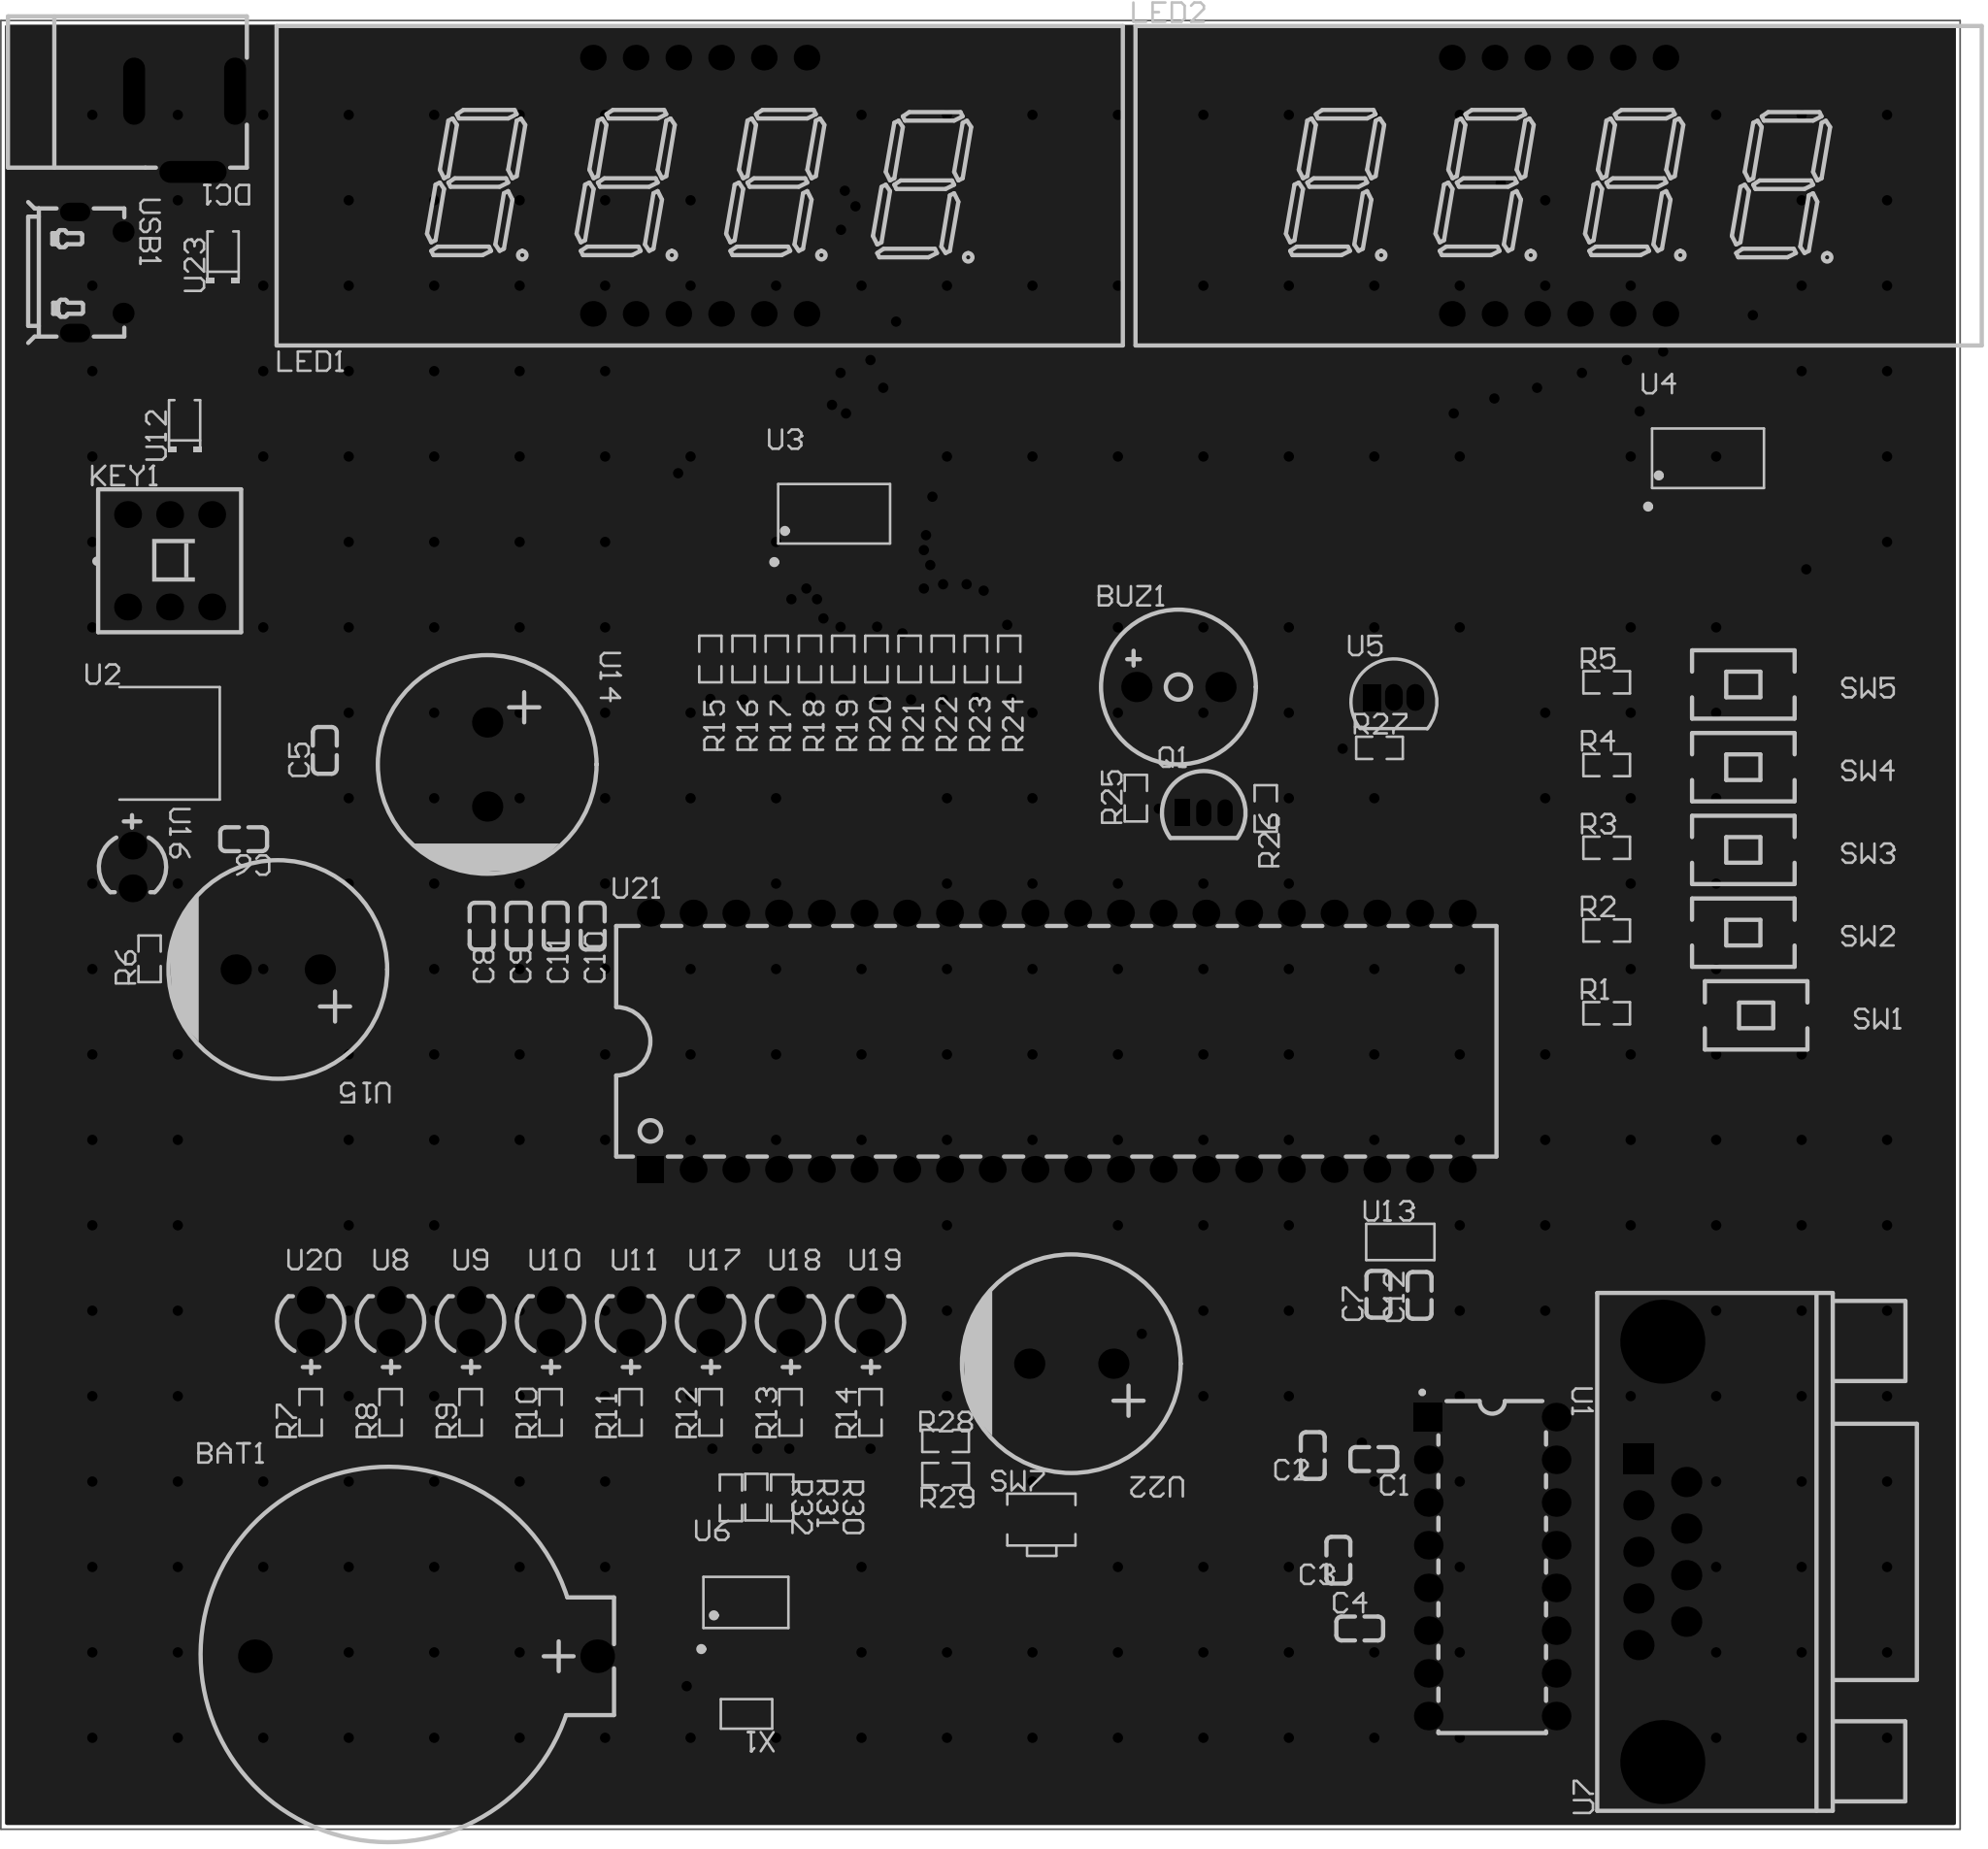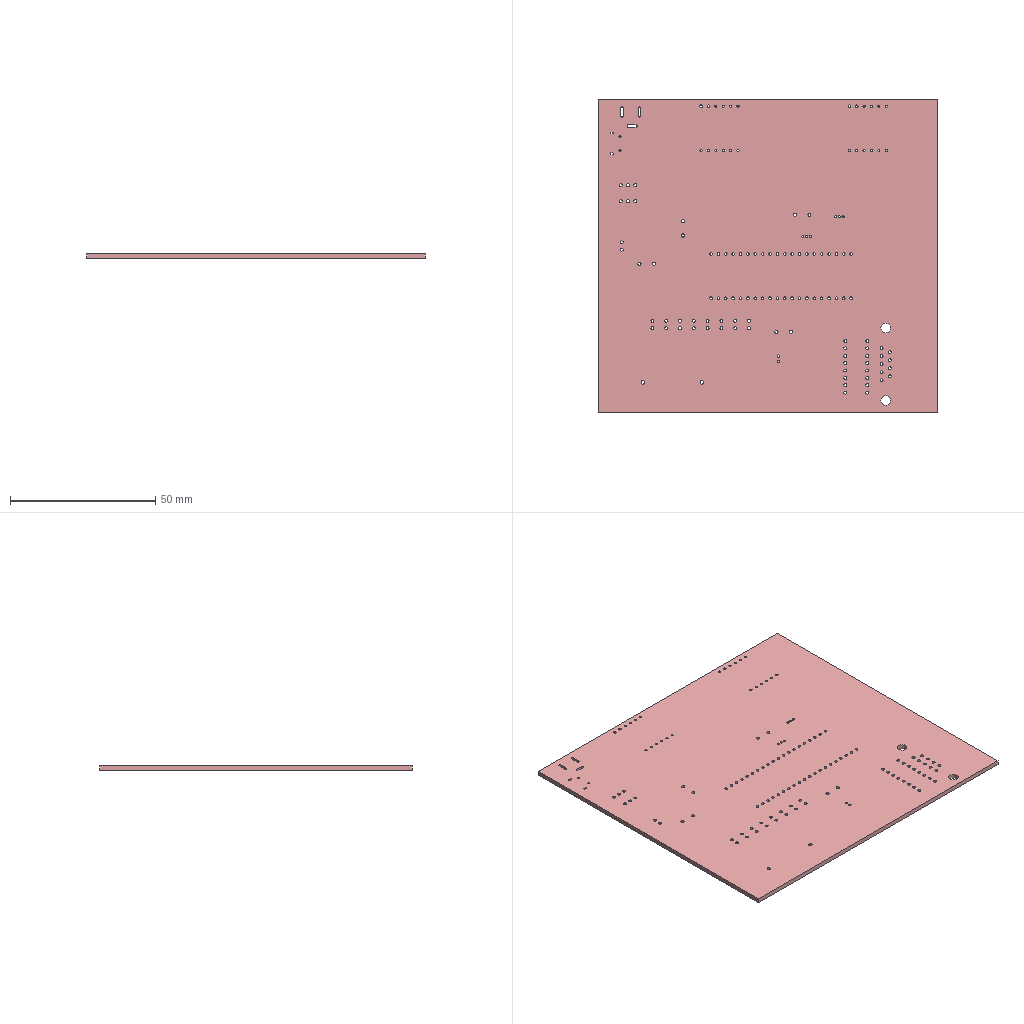Circuit board layout | Altium Designer | box 116.5 x 107.6 x 1.6 mm
Layer stack:
# Altium Designer layer stack of  (unit mm; dielectric type: 0 none, 1 core, 2 prepreg, 3 surface material)
index,name,kind,layer,copper_thickness_mm,dielectric_type,dielectric_thickness_mm,dielectric_material,dielectric_constant
0,Top Paste Mask Layer,other,,,,,,
1,Top Silkscreen Layer,other,,,,,,
2,Top Solder Mask Layer,dielectric,,,3,0.01,,3.3
3,Top Layer,copper,Top Layer,0.035,,,,
4,Dielectric1,dielectric,,,3,1.51,FR4,4.5
5,Bottom Layer,copper,Bottom Layer,0.035,,,,
6,Bottom Solder Mask Layer,dielectric,,,3,0.01,,3.3
7,Bottom Silkscreen Layer,other,,,,,,
8,Bottom Paste Mask Layer,other,,,,,,
# drill layer pairs: low layer,high layer
drill_pair,Top Layer,Bottom Layer
Part placement:
Designator,Comment,Layer,Footprint,Center-X(mm),Center-Y(mm),Rotation
BUZ1,Buzzer,TopLayer,BUZ-TH_BD9.0-P5.00-D0.6-FD,160.419,151.371,0
C1,104,TopLayer,C0603,172.032,105.452,180
C2,4.7uF,TopLayer,C0603,168.402,105.664,90
C3,4.7uF,TopLayer,C0603,169.926,99.441,90
C4,4.7uF,TopLayer,C0603,171.196,95.377,0
C5,4.7uF,TopLayer,C0603,109.68,147.6,90
C6,4.7uF,TopLayer,C0603,104.857,142.317,180
C7,100nF,TopLayer,C0603,172.308,115.254,90
C8,4.7uF,TopLayer,C0603,118.999,137.15,90
C9,4.7uF,TopLayer,C0603,121.2,137.15,90
C10,4.7uF,TopLayer,C0603,125.603,137.15,90
C11,4.7uF,TopLayer,C0603,123.402,137.15,90
C12,100nF,TopLayer,C0603,174.752,115.189,90
LED1,FJ5461AB,TopLayer,LED-SEG-TH_12P-L50.4-W19.0-P2.54-S15.24-BL,131.964,181.182,0
LED2,FJ5461AB,TopLayer,LED-SEG-TH_12P-L50.4-W19.0-P2.54-S15.24-BL,183.018,181.182,0
Q1,2SC945,TopLayer,TO-92-3_L4.9-W3.7-P1.27-L,161.925,143.891,0
R1,48.7Ω,TopLayer,R0603,185.875,131.969,0
R2,48.7Ω,TopLayer,R0603,185.875,136.888,0
R3,48.7Ω,TopLayer,R0603,185.875,141.808,0
R4,48.7Ω,TopLayer,R0603,185.875,146.728,0
R5,48.7Ω,TopLayer,R0603,185.875,151.648,0
R6,10K,TopLayer,R0603,99.266,135.205,90
R7,10K,TopLayer,R0603,108.837,108.233,90
R8,10K,TopLayer,R0603,113.591,108.233,90
R9,10K,TopLayer,R0603,118.345,108.233,90
R10,10K,TopLayer,R0603,123.099,108.233,90
R11,10K,TopLayer,R0603,127.853,108.233,90
R12,10K,TopLayer,R0603,132.607,108.233,90
R13,10K,TopLayer,R0603,137.361,108.233,90
R14,10K,TopLayer,R0603,142.115,108.233,90
R15,10K,TopLayer,R0603,132.597,153.035,90
R16,10K,TopLayer,R0603,134.57,153.035,90
R17,10K,TopLayer,R0603,136.544,153.035,90
R18,10K,TopLayer,R0603,138.518,153.035,90
R19,10K,TopLayer,R0603,140.491,153.035,90
R20,10K,TopLayer,R0603,142.465,153.035,90
R21,10K,TopLayer,R0603,144.438,153.035,90
R22,10K,TopLayer,R0603,146.412,153.035,90
R23,10K,TopLayer,R0603,148.386,153.035,90
R24,10K,TopLayer,R0603,150.359,153.035,90
R25,50,TopLayer,R0603,157.888,144.759,90
R26,1K,TopLayer,R0603,165.608,144.145,90
R27,10K,TopLayer,R0603,172.371,147.751,0
R28,10K,TopLayer,R0603,146.578,106.535,180
R29,10K,TopLayer,R0603,146.578,104.562,0
SW1,SW_PB_ESW_1,TopLayer,KEY-SMD_L6.1-W3.8-LS8.0,194.758,131.841,0
SW2,SW_PB_ESW_1,TopLayer,KEY-SMD_L6.1-W3.8-LS8.0,193.996,136.761,0
SW3,SW_PB_ESW_1,TopLayer,KEY-SMD_L6.1-W3.8-LS8.0,193.996,141.681,0
SW4,SW_PB_ESW_1,TopLayer,KEY-SMD_L6.1-W3.8-LS8.0,193.996,146.601,0
SW5,SW_PB_ESW_1,TopLayer,KEY-SMD_L6.1-W3.8-LS8.0,193.996,151.521,0
SW7,YD-3410,TopLayer,SW-SMD_L3.9-W2.9-LS4.8-EH-A,152.273,101.854,0
U1,MAX232AEJE,TopLayer,PDIP-16_L19.3-W6.5-P2.54-LS7.6-BL,179.07,99.06,270
U2,LM1117IDT-5.0,TopLayer,TO-252-2_L6.6-W6.1-P4.57-LS9.7-BR-CW,102.055,148.018,0
U3,74HC573PW/AU118,TopLayer,TSSOP-20_L6.5-W4.4-P0.65-LS6.4-BL,139.954,161.671,0
U4,74HC573PW/AU118,TopLayer,TSSOP-20_L6.5-W4.4-P0.65-LS6.4-BL,191.897,164.973,0
U5,DS18B20+T&R-HX,TopLayer,TO-92-3_L5.1-W4.1-P1.27-L-1,173.228,150.749,0
U6,DS1302Z+T&R-TUDI,TopLayer,SOIC-8_L4.9-W3.9-P1.27-LS6.0-BL,134.71,96.927,0
U7,DB9F,TopLayer,DB9-TH_DB9F_C9900018961,189.182,99.934,90
U8,LED,TopLayer,LED-TH_BD4.0-P2.54-FD_RED,113.591,113.637,90
U9,LED,TopLayer,LED-TH_BD4.0-P2.54-FD_RED,118.345,113.637,90
U10,LED,TopLayer,LED-TH_BD4.0-P2.54-FD_RED,123.099,113.637,90
U11,LED,TopLayer,LED-TH_BD4.0-P2.54-FD_RED,127.853,113.637,90
U12,IN5819,TopLayer,SOD-123_L2.7-W1.7-LS3.8-RD,101.346,167.005,90
U13,2.768KHz,TopLayer,CRYSTAL-SMD_L3.2-W1.5-1,173.609,118.364,0
U14,CE63V1000uF13*25,TopLayer,CAP-TH_BD13.0-P5.00-D0.6-FD,119.332,146.762,270
U15,10uF,TopLayer,CAP-TH_BD13.0-P5.00-D0.6-FD,106.886,134.57,180
U16,LED,TopLayer,LED-TH_BD4.0-P2.54-FD_RED,98.25,140.666,270
U17,LED,TopLayer,LED-TH_BD4.0-P2.54-FD_RED,132.607,113.637,90
U18,LED,TopLayer,LED-TH_BD4.0-P2.54-FD_RED,137.361,113.637,90
U19,LED,TopLayer,LED-TH_BD4.0-P2.54-FD_RED,142.115,113.637,90
U20,LED,TopLayer,LED-TH_BD4.0-P2.54-FD_RED,108.837,113.637,90
U21,STC89C53RC-40I-PDIP40,TopLayer,DIP-40_L52.0-W13.7-P2.54-LS15.2-BL,153.162,130.302,0
U22,CE63V1000uF13*25,TopLayer,CAP-TH_BD13.0-P5.00-D0.6-FD,154.051,111.125,180
USB1,MICRO-USB-1,TopLayer,MICRO-USB-SMD_C9900008946,96.266,176.022,270
BAT1,CR2032-2-1,TopLayer,BAT-TH_CR2032-2-1,115.697,93.726,0
DC1,,TopLayer,DC-2.0,101.346,184.404,180
KEY1,Non-latching switch 8.5×8.5 silent,TopLayer,SW-TH_6P-L8.5-W8.5-P2.54,100.457,158.877,0
R30,4.7K,TopLayer,R0603,136.869,103.15,270
R31,4.7K,TopLayer,R0603,135.325,103.191,270
R32,4.7K,TopLayer,R0603,133.821,103.15,270
U23,IN5819,TopLayer,SOD-123_L2.7-W1.7-LS3.8-RD,103.632,177.038,90
X1,32.768K,TopLayer,OSC-SMD_L2.0-W1.2,134.747,90.297,180
Pad and via stacks:
# Altium Designer via and pad stacks of  (unit mm). Each distinct definition once, with the count of objects using it.
# via: kind,start_layer,end_layer,hole_mm,diameter_mm,mode(0 simple;1 top-mid-bottom;2 full stack),diameter_per_layer,count,example_net
# pad: kind,layer,hole_mm,hole_type(0 round;1 square;2 slot),plating,top_size,top_shape(1 round;2 rect;3 octagon;9 rounded rect),mid_size,bottom_size,mode,footprint,size_per_layer,count,example
pad,Multi-Layer,1,0,plated,1.8x1.8,1,1.8x1.8,1.8x1.8,0,BUZ-TH_BD9.0-P5.00-D0.6-FD,,2,BUZ1.1
pad,Multi-Layer,0.9144,0,plated,1.524x1.524,1,1.524x1.524,1.524x1.524,0,LED-SEG-TH_12P-L50.4-W19.0-P2.54-S15.24-BL,,4,LED1.12
pad,Multi-Layer,0.762,0,plated,1.524x1.524,1,1.524x1.524,1.524x1.524,0,LED-SEG-TH_12P-L50.4-W19.0-P2.54-S15.24-BL,,20,LED1.10
pad,Multi-Layer,0.7,0,plated,0.9x1.6,1,0.9x1.6,0.9x1.6,0,TO-92-3_L4.9-W3.7-P1.27-L,,2,Q1.3
pad,Multi-Layer,0.7,0,plated,0.9x1.6,2,0.9x1.6,0.9x1.6,0,TO-92-3_L4.9-W3.7-P1.27-L,,1,Q1.1
pad,Multi-Layer,1,0,plated,1.7x1.7,2,1.7x1.7,1.7x1.7,0,PDIP-16_L19.3-W6.5-P2.54-LS7.6-BL,,1,U1.1
pad,Multi-Layer,1,0,plated,1.7x1.7,1,1.7x1.7,1.7x1.7,0,PDIP-16_L19.3-W6.5-P2.54-LS7.6-BL,,15,U1.2
pad,Multi-Layer,0.75,0,plated,1.05x1.6,2,1.05x1.6,1.05x1.6,0,TO-92-3_L5.1-W4.1-P1.27-L-1,,1,U5.1
pad,Multi-Layer,0.75,0,plated,1.05x1.6,1,1.05x1.6,1.05x1.6,0,TO-92-3_L5.1-W4.1-P1.27-L-1,,2,U5.2
pad,Multi-Layer,3.25,0,plated,5x5,1,5x5,5x5,0,DB9-TH_DB9F_C9900018961,,2,U7.10
pad,Multi-Layer,1.05,0,plated,1.8x1.8,1,1.8x1.8,1.8x1.8,0,DB9-TH_DB9F_C9900018961,,8,U7.6
pad,Multi-Layer,1.05,0,plated,1.8x1.8,2,1.8x1.8,1.8x1.8,0,DB9-TH_DB9F_C9900018961,,1,U7.1
pad,Multi-Layer,1,0,plated,1.651x1.651,1,1.651x1.651,1.651x1.651,0,LED-TH_BD4.0-P2.54-FD_RED,,18,U8.2
pad,Multi-Layer,1.1,0,plated,1.8x1.8,1,1.8x1.8,1.8x1.8,0,CAP-TH_BD13.0-P5.00-D0.6-FD,,6,U14.1
pad,Multi-Layer,0.889,0,plated,1.6x1.6,1,1.6x1.6,1.6x1.6,0,DIP-40_L52.0-W13.7-P2.54-LS15.2-BL,,39,U21.31
pad,Multi-Layer,0.889,0,plated,1.6x1.6,2,1.6x1.6,1.6x1.6,0,DIP-40_L52.0-W13.7-P2.54-LS15.2-BL,,1,U21.1
pad,Multi-Layer,0.7,0,plated,1.25x1.25,1,1.25x1.25,1.25x1.25,0,MICRO-USB-SMD_C9900008946,,2,USB1.6
pad,Multi-Layer,0.6,2,plated,1.1x1.8,1,1.1x1.8,1.1x1.8,0,MICRO-USB-SMD_C9900008946,,2,USB1.6
pad,Multi-Layer,1.2,0,plated,2x2,1,2x2,2x2,0,BAT-TH_CR2032-2-1,,2,BAT1.2
pad,Multi-Layer,0.8001,2,plated,4x1.3,1,4x1.3,4x1.3,0,DC-2.0,,3,DC1.2
pad,Multi-Layer,1,0,plated,1.6x1.6,1,1.6x1.6,1.6x1.6,0,SW-TH_6P-L8.5-W8.5-P2.54,,6,KEY1.4
pad,Top Layer,0,0,plated,0.8x0.9,2,0.8x0.9,0.8x0.9,0,C0603,,24,C1.2
pad,Top Layer,0,0,plated,0.8065x0.864,2,0.8065x0.864,0.8065x0.864,0,R0603,,64,R1.2
pad,Top Layer,0,0,plated,2x1.2,2,2x1.2,2x1.2,0,KEY-SMD_L6.1-W3.8-LS8.0,,10,SW1.1
pad,Top Layer,0,0,plated,1.23x1.5,2,1.23x1.5,1.23x1.5,0,SW-SMD_L3.9-W2.9-LS4.8-EH-A,,2,SW7.2
pad,Top Layer,0,0,plated,6.2x5.8,2,6.2x5.8,6.2x5.8,0,TO-252-2_L6.6-W6.1-P4.57-LS9.7-BR-CW,,1,U2.2
pad,Top Layer,0,0,plated,3x1.6,2,3x1.6,3x1.6,0,TO-252-2_L6.6-W6.1-P4.57-LS9.7-BR-CW,,2,U2.3
pad,Top Layer,0,0,plated,0.364x1.742,1,0.364x1.742,0.364x1.742,0,TSSOP-20_L6.5-W4.4-P0.65-LS6.4-BL,,40,U3.1
pad,Top Layer,0,0,plated,0.588x2.045,1,0.588x2.045,0.588x2.045,0,SOIC-8_L4.9-W3.9-P1.27-LS6.0-BL,,8,U6.5
pad,Top Layer,0,0,plated,0.91x0.84,2,0.91x0.84,0.91x0.84,0,SOD-123_L2.7-W1.7-LS3.8-RD,,4,U12.1
pad,Top Layer,0,0,plated,1.05x1.7,2,1.05x1.7,1.05x1.7,0,CRYSTAL-SMD_L3.2-W1.5-1,,2,U13.2
pad,Top Layer,0,0,plated,1.35x0.4,2,1.35x0.4,1.35x0.4,0,MICRO-USB-SMD_C9900008946,,5,USB1.1
pad,Top Layer,0,0,plated,0.7x1.3,2,0.7x1.3,0.7x1.3,0,OSC-SMD_L2.0-W1.2,,2,X1.1
via,Top Layer,Bottom Layer,0.3048,0.61,0,,351,F
Copper pours:
name,layer,net,type(0 solid;1 hatched;2 none)
Top Layer-GND,Top Layer,GND,0
Bottom Layer-GND,Bottom Layer,GND,0